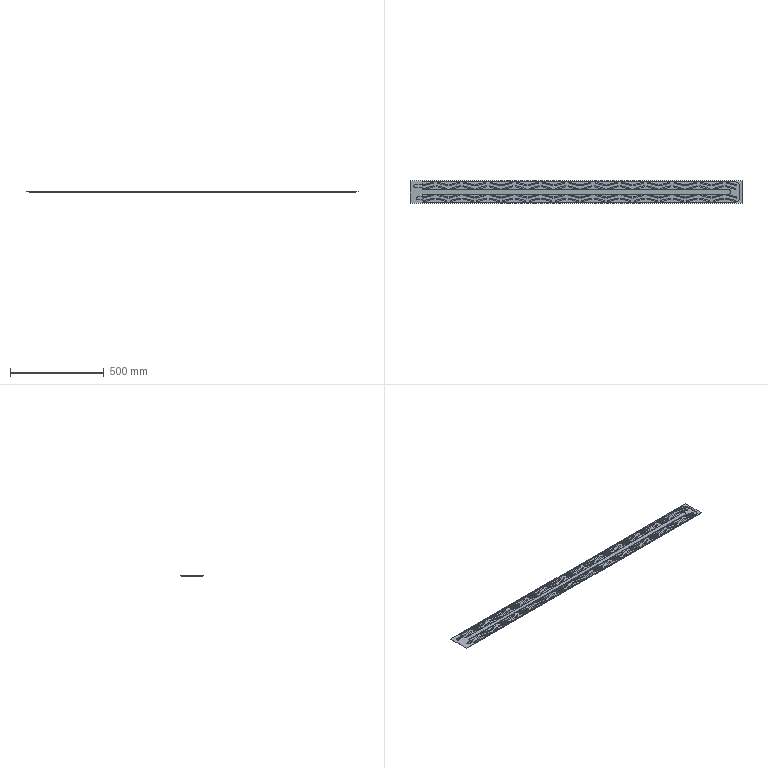Part | SolidWorks | features ICE 4, BaseBody 1, LPattern 1, MirrorPattern 1 | 1 solid | 1200 faces | box 1768 x 120 x 5 mm | volume 284579 mm3 | plane 612 | cylinder 588 | commonest cylinder face diameters 4 x288 6 x288 12 x2 14 x2 18 x2 20 x2